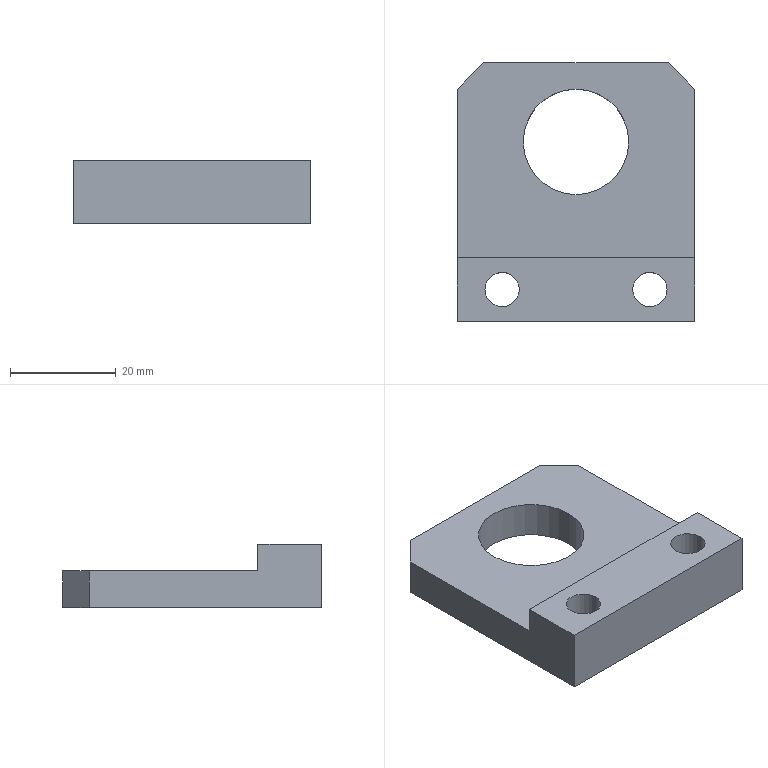Part | STEP file | magnetic tile top shaft cylinder seat 2 | 1 solid | 16 faces | box 45 x 49 x 12 mm | volume 14964 mm3 | plane 10 | cylinder 6 | commonest cylinder face diameters 6.5 x4 20 x2
STEP:
#1=CARTESIAN_POINT('',(0.,0.,0.));
#2=DIRECTION('',(0.,0.,1.));
#3=DIRECTION('',(1.,0.,0.));
#4=AXIS2_PLACEMENT_3D('',#1,#2,#3);
#5=CARTESIAN_POINT('',(10.75,-28.,12.));
#6=VERTEX_POINT('',#5);
#7=CARTESIAN_POINT('',(10.75,-28.,0.));
#8=VERTEX_POINT('',#7);
#9=CARTESIAN_POINT('',(10.75,-28.,12.));
#10=DIRECTION('',(0.,0.,-1.));
#11=VECTOR('',#10,1.);
#12=LINE('',#9,#11);
#13=CARTESIAN_POINT('',(14.,-28.,12.));
#14=DIRECTION('',(0.,0.,-1.));
#15=DIRECTION('',(-1.,0.,0.));
#16=AXIS2_PLACEMENT_3D('',#13,#14,#15);
#17=CYLINDRICAL_SURFACE('',#16,3.25);
#18=CARTESIAN_POINT('',(6.283,0.));
#19=DIRECTION('',(0.,1.));
#20=VECTOR('',#19,1.);
#21=LINE('',#18,#20);
#22=(GEOMETRIC_REPRESENTATION_CONTEXT(2)PARAMETRIC_REPRESENTATION_CONTEXT()REPRESENTATION_CONTEXT('',''));
#23=DEFINITIONAL_REPRESENTATION('',(#21),#22);
#24=PCURVE('',#17,#23);
#25=CARTESIAN_POINT('',(14.,-28.,12.));
#26=DIRECTION('',(0.,0.,-1.));
#27=DIRECTION('',(-1.,0.,0.));
#28=AXIS2_PLACEMENT_3D('',#25,#26,#27);
#29=CYLINDRICAL_SURFACE('',#28,3.25);
#30=CARTESIAN_POINT('',(0.,0.));
#31=DIRECTION('',(0.,1.));
#32=VECTOR('',#31,1.);
#33=LINE('',#30,#32);
#34=(GEOMETRIC_REPRESENTATION_CONTEXT(2)PARAMETRIC_REPRESENTATION_CONTEXT()REPRESENTATION_CONTEXT('',''));
#35=DEFINITIONAL_REPRESENTATION('',(#33),#34);
#36=PCURVE('',#29,#35);
#37=SURFACE_CURVE('',#12,(#24,#36),.PCURVE_S1.);
#38=EDGE_CURVE('',#6,#8,#37,.T.);
#39=ORIENTED_EDGE('',*,*,#38,.T.);
#40=CARTESIAN_POINT('',(17.25,-28.,0.));
#41=VERTEX_POINT('',#40);
#42=CARTESIAN_POINT('',(14.,-28.,0.));
#43=DIRECTION('',(0.,0.,-1.));
#44=DIRECTION('',(-1.,0.,0.));
#45=AXIS2_PLACEMENT_3D('',#42,#43,#44);
#46=CIRCLE('',#45,3.25);
#47=CARTESIAN_POINT('',(0.,12.));
#48=DIRECTION('',(1.,0.));
#49=VECTOR('',#48,1.);
#50=LINE('',#47,#49);
#51=(GEOMETRIC_REPRESENTATION_CONTEXT(2)PARAMETRIC_REPRESENTATION_CONTEXT()REPRESENTATION_CONTEXT('',''));
#52=DEFINITIONAL_REPRESENTATION('',(#50),#51);
#53=PCURVE('',#17,#52);
#54=CARTESIAN_POINT('',(-22.5,-34.,0.));
#55=DIRECTION('',(0.,0.,1.));
#56=DIRECTION('',(1.,0.,0.));
#57=AXIS2_PLACEMENT_3D('',#54,#55,#56);
#58=PLANE('',#57);
#59=CARTESIAN_POINT('',(33.25,6.));
#60=CARTESIAN_POINT('',(33.25,11.629));
#61=CARTESIAN_POINT('',(38.125,8.815));
#62=CARTESIAN_POINT('',(43.,6.));
#63=CARTESIAN_POINT('',(38.125,3.185));
#64=CARTESIAN_POINT('',(33.25,0.3708));
#65=CARTESIAN_POINT('',(33.25,6.));
#66=(BOUNDED_CURVE()B_SPLINE_CURVE(2,(#59,#60,#61,#62,#63,#64,#65),.UNSPECIFIED.,.T.,.F.)B_SPLINE_CURVE_WITH_KNOTS((1,2,2,2,2,1),(-2.094,0.,2.094,4.189,6.283,8.378),.UNSPECIFIED.)CURVE()GEOMETRIC_REPRESENTATION_ITEM()RATIONAL_B_SPLINE_CURVE((1.,0.5,1.,0.5,1.,0.5,1.))REPRESENTATION_ITEM(''));
#67=(GEOMETRIC_REPRESENTATION_CONTEXT(2)PARAMETRIC_REPRESENTATION_CONTEXT()REPRESENTATION_CONTEXT('',''));
#68=DEFINITIONAL_REPRESENTATION('',(#66),#67);
#69=PCURVE('',#58,#68);
#70=SURFACE_CURVE('',#46,(#53,#69),.PCURVE_S1.);
#71=EDGE_CURVE('',#41,#8,#70,.T.);
#72=ORIENTED_EDGE('',*,*,#71,.F.);
#73=CARTESIAN_POINT('',(17.25,-28.,12.));
#74=VERTEX_POINT('',#73);
#75=CARTESIAN_POINT('',(17.25,-28.,12.));
#76=DIRECTION('',(0.,0.,-1.));
#77=VECTOR('',#76,1.);
#78=LINE('',#75,#77);
#79=CARTESIAN_POINT('',(3.142,0.));
#80=DIRECTION('',(0.,1.));
#81=VECTOR('',#80,1.);
#82=LINE('',#79,#81);
#83=(GEOMETRIC_REPRESENTATION_CONTEXT(2)PARAMETRIC_REPRESENTATION_CONTEXT()REPRESENTATION_CONTEXT('',''));
#84=DEFINITIONAL_REPRESENTATION('',(#82),#83);
#85=PCURVE('',#17,#84);
#86=CARTESIAN_POINT('',(3.142,0.));
#87=DIRECTION('',(0.,1.));
#88=VECTOR('',#87,1.);
#89=LINE('',#86,#88);
#90=(GEOMETRIC_REPRESENTATION_CONTEXT(2)PARAMETRIC_REPRESENTATION_CONTEXT()REPRESENTATION_CONTEXT('',''));
#91=DEFINITIONAL_REPRESENTATION('',(#89),#90);
#92=PCURVE('',#29,#91);
#93=SURFACE_CURVE('',#78,(#85,#92),.PCURVE_S1.);
#94=EDGE_CURVE('',#74,#41,#93,.T.);
#95=ORIENTED_EDGE('',*,*,#94,.F.);
#96=CARTESIAN_POINT('',(14.,-28.,12.));
#97=DIRECTION('',(0.,0.,-1.));
#98=DIRECTION('',(-1.,0.,0.));
#99=AXIS2_PLACEMENT_3D('',#96,#97,#98);
#100=CIRCLE('',#99,3.25);
#101=CARTESIAN_POINT('',(0.,0.));
#102=DIRECTION('',(1.,0.));
#103=VECTOR('',#102,1.);
#104=LINE('',#101,#103);
#105=(GEOMETRIC_REPRESENTATION_CONTEXT(2)PARAMETRIC_REPRESENTATION_CONTEXT()REPRESENTATION_CONTEXT('',''));
#106=DEFINITIONAL_REPRESENTATION('',(#104),#105);
#107=PCURVE('',#17,#106);
#108=CARTESIAN_POINT('',(-22.5,-34.,12.));
#109=DIRECTION('',(0.,0.,1.));
#110=DIRECTION('',(1.,0.,0.));
#111=AXIS2_PLACEMENT_3D('',#108,#109,#110);
#112=PLANE('',#111);
#113=CARTESIAN_POINT('',(33.25,6.));
#114=CARTESIAN_POINT('',(33.25,11.629));
#115=CARTESIAN_POINT('',(38.125,8.815));
#116=CARTESIAN_POINT('',(43.,6.));
#117=CARTESIAN_POINT('',(38.125,3.185));
#118=CARTESIAN_POINT('',(33.25,0.3708));
#119=CARTESIAN_POINT('',(33.25,6.));
#120=(BOUNDED_CURVE()B_SPLINE_CURVE(2,(#113,#114,#115,#116,#117,#118,#119),.UNSPECIFIED.,.T.,.F.)B_SPLINE_CURVE_WITH_KNOTS((1,2,2,2,2,1),(-2.094,0.,2.094,4.189,6.283,8.378),.UNSPECIFIED.)CURVE()GEOMETRIC_REPRESENTATION_ITEM()RATIONAL_B_SPLINE_CURVE((1.,0.5,1.,0.5,1.,0.5,1.))REPRESENTATION_ITEM(''));
#121=(GEOMETRIC_REPRESENTATION_CONTEXT(2)PARAMETRIC_REPRESENTATION_CONTEXT()REPRESENTATION_CONTEXT('',''));
#122=DEFINITIONAL_REPRESENTATION('',(#120),#121);
#123=PCURVE('',#112,#122);
#124=SURFACE_CURVE('',#100,(#107,#123),.PCURVE_S1.);
#125=EDGE_CURVE('',#74,#6,#124,.T.);
#126=ORIENTED_EDGE('',*,*,#125,.T.);
#127=EDGE_LOOP('',(#39,#72,#95,#126));
#128=FACE_BOUND('',#127,.F.);
#129=ADVANCED_FACE('',(#128),#17,.F.);
#130=CARTESIAN_POINT('',(-17.25,-28.,12.));
#131=VERTEX_POINT('',#130);
#132=CARTESIAN_POINT('',(-17.25,-28.,0.));
#133=VERTEX_POINT('',#132);
#134=CARTESIAN_POINT('',(-17.25,-28.,12.));
#135=DIRECTION('',(0.,0.,-1.));
#136=VECTOR('',#135,1.);
#137=LINE('',#134,#136);
#138=CARTESIAN_POINT('',(-14.,-28.,12.));
#139=DIRECTION('',(0.,0.,-1.));
#140=DIRECTION('',(-1.,0.,0.));
#141=AXIS2_PLACEMENT_3D('',#138,#139,#140);
#142=CYLINDRICAL_SURFACE('',#141,3.25);
#143=CARTESIAN_POINT('',(6.283,0.));
#144=DIRECTION('',(0.,1.));
#145=VECTOR('',#144,1.);
#146=LINE('',#143,#145);
#147=(GEOMETRIC_REPRESENTATION_CONTEXT(2)PARAMETRIC_REPRESENTATION_CONTEXT()REPRESENTATION_CONTEXT('',''));
#148=DEFINITIONAL_REPRESENTATION('',(#146),#147);
#149=PCURVE('',#142,#148);
#150=CARTESIAN_POINT('',(-14.,-28.,12.));
#151=DIRECTION('',(0.,0.,-1.));
#152=DIRECTION('',(-1.,0.,0.));
#153=AXIS2_PLACEMENT_3D('',#150,#151,#152);
#154=CYLINDRICAL_SURFACE('',#153,3.25);
#155=CARTESIAN_POINT('',(0.,0.));
#156=DIRECTION('',(0.,1.));
#157=VECTOR('',#156,1.);
#158=LINE('',#155,#157);
#159=(GEOMETRIC_REPRESENTATION_CONTEXT(2)PARAMETRIC_REPRESENTATION_CONTEXT()REPRESENTATION_CONTEXT('',''));
#160=DEFINITIONAL_REPRESENTATION('',(#158),#159);
#161=PCURVE('',#154,#160);
#162=SURFACE_CURVE('',#137,(#149,#161),.PCURVE_S1.);
#163=EDGE_CURVE('',#131,#133,#162,.T.);
#164=ORIENTED_EDGE('',*,*,#163,.T.);
#165=CARTESIAN_POINT('',(-10.75,-28.,0.));
#166=VERTEX_POINT('',#165);
#167=CARTESIAN_POINT('',(-14.,-28.,0.));
#168=DIRECTION('',(0.,0.,-1.));
#169=DIRECTION('',(-1.,0.,0.));
#170=AXIS2_PLACEMENT_3D('',#167,#168,#169);
#171=CIRCLE('',#170,3.25);
#172=CARTESIAN_POINT('',(0.,12.));
#173=DIRECTION('',(1.,0.));
#174=VECTOR('',#173,1.);
#175=LINE('',#172,#174);
#176=(GEOMETRIC_REPRESENTATION_CONTEXT(2)PARAMETRIC_REPRESENTATION_CONTEXT()REPRESENTATION_CONTEXT('',''));
#177=DEFINITIONAL_REPRESENTATION('',(#175),#176);
#178=PCURVE('',#142,#177);
#179=CARTESIAN_POINT('',(5.25,6.));
#180=CARTESIAN_POINT('',(5.25,11.629));
#181=CARTESIAN_POINT('',(10.125,8.815));
#182=CARTESIAN_POINT('',(15.,6.));
#183=CARTESIAN_POINT('',(10.125,3.185));
#184=CARTESIAN_POINT('',(5.25,0.3708));
#185=CARTESIAN_POINT('',(5.25,6.));
#186=(BOUNDED_CURVE()B_SPLINE_CURVE(2,(#179,#180,#181,#182,#183,#184,#185),.UNSPECIFIED.,.T.,.F.)B_SPLINE_CURVE_WITH_KNOTS((1,2,2,2,2,1),(-2.094,0.,2.094,4.189,6.283,8.378),.UNSPECIFIED.)CURVE()GEOMETRIC_REPRESENTATION_ITEM()RATIONAL_B_SPLINE_CURVE((1.,0.5,1.,0.5,1.,0.5,1.))REPRESENTATION_ITEM(''));
#187=(GEOMETRIC_REPRESENTATION_CONTEXT(2)PARAMETRIC_REPRESENTATION_CONTEXT()REPRESENTATION_CONTEXT('',''));
#188=DEFINITIONAL_REPRESENTATION('',(#186),#187);
#189=PCURVE('',#58,#188);
#190=SURFACE_CURVE('',#171,(#178,#189),.PCURVE_S1.);
#191=EDGE_CURVE('',#166,#133,#190,.T.);
#192=ORIENTED_EDGE('',*,*,#191,.F.);
#193=CARTESIAN_POINT('',(-10.75,-28.,12.));
#194=VERTEX_POINT('',#193);
#195=CARTESIAN_POINT('',(-10.75,-28.,12.));
#196=DIRECTION('',(0.,0.,-1.));
#197=VECTOR('',#196,1.);
#198=LINE('',#195,#197);
#199=CARTESIAN_POINT('',(3.142,0.));
#200=DIRECTION('',(0.,1.));
#201=VECTOR('',#200,1.);
#202=LINE('',#199,#201);
#203=(GEOMETRIC_REPRESENTATION_CONTEXT(2)PARAMETRIC_REPRESENTATION_CONTEXT()REPRESENTATION_CONTEXT('',''));
#204=DEFINITIONAL_REPRESENTATION('',(#202),#203);
#205=PCURVE('',#142,#204);
#206=CARTESIAN_POINT('',(3.142,0.));
#207=DIRECTION('',(0.,1.));
#208=VECTOR('',#207,1.);
#209=LINE('',#206,#208);
#210=(GEOMETRIC_REPRESENTATION_CONTEXT(2)PARAMETRIC_REPRESENTATION_CONTEXT()REPRESENTATION_CONTEXT('',''));
#211=DEFINITIONAL_REPRESENTATION('',(#209),#210);
#212=PCURVE('',#154,#211);
#213=SURFACE_CURVE('',#198,(#205,#212),.PCURVE_S1.);
#214=EDGE_CURVE('',#194,#166,#213,.T.);
#215=ORIENTED_EDGE('',*,*,#214,.F.);
#216=CARTESIAN_POINT('',(-14.,-28.,12.));
#217=DIRECTION('',(0.,0.,-1.));
#218=DIRECTION('',(-1.,0.,0.));
#219=AXIS2_PLACEMENT_3D('',#216,#217,#218);
#220=CIRCLE('',#219,3.25);
#221=CARTESIAN_POINT('',(0.,0.));
#222=DIRECTION('',(1.,0.));
#223=VECTOR('',#222,1.);
#224=LINE('',#221,#223);
#225=(GEOMETRIC_REPRESENTATION_CONTEXT(2)PARAMETRIC_REPRESENTATION_CONTEXT()REPRESENTATION_CONTEXT('',''));
#226=DEFINITIONAL_REPRESENTATION('',(#224),#225);
#227=PCURVE('',#142,#226);
#228=CARTESIAN_POINT('',(5.25,6.));
#229=CARTESIAN_POINT('',(5.25,11.629));
#230=CARTESIAN_POINT('',(10.125,8.815));
#231=CARTESIAN_POINT('',(15.,6.));
#232=CARTESIAN_POINT('',(10.125,3.185));
#233=CARTESIAN_POINT('',(5.25,0.3708));
#234=CARTESIAN_POINT('',(5.25,6.));
#235=(BOUNDED_CURVE()B_SPLINE_CURVE(2,(#228,#229,#230,#231,#232,#233,#234),.UNSPECIFIED.,.T.,.F.)B_SPLINE_CURVE_WITH_KNOTS((1,2,2,2,2,1),(-2.094,0.,2.094,4.189,6.283,8.378),.UNSPECIFIED.)CURVE()GEOMETRIC_REPRESENTATION_ITEM()RATIONAL_B_SPLINE_CURVE((1.,0.5,1.,0.5,1.,0.5,1.))REPRESENTATION_ITEM(''));
#236=(GEOMETRIC_REPRESENTATION_CONTEXT(2)PARAMETRIC_REPRESENTATION_CONTEXT()REPRESENTATION_CONTEXT('',''));
#237=DEFINITIONAL_REPRESENTATION('',(#235),#236);
#238=PCURVE('',#112,#237);
#239=SURFACE_CURVE('',#220,(#227,#238),.PCURVE_S1.);
#240=EDGE_CURVE('',#194,#131,#239,.T.);
#241=ORIENTED_EDGE('',*,*,#240,.T.);
#242=EDGE_LOOP('',(#164,#192,#215,#241));
#243=FACE_BOUND('',#242,.F.);
#244=ADVANCED_FACE('',(#243),#142,.F.);
#245=CARTESIAN_POINT('',(-10.,0.,7.));
#246=VERTEX_POINT('',#245);
#247=CARTESIAN_POINT('',(-10.,0.,0.));
#248=VERTEX_POINT('',#247);
#249=CARTESIAN_POINT('',(-10.,0.,12.));
#250=DIRECTION('',(0.,0.,-1.));
#251=VECTOR('',#250,1.);
#252=LINE('',#249,#251);
#253=CARTESIAN_POINT('',(0.,0.,12.));
#254=DIRECTION('',(0.,0.,-1.));
#255=DIRECTION('',(-1.,0.,0.));
#256=AXIS2_PLACEMENT_3D('',#253,#254,#255);
#257=CYLINDRICAL_SURFACE('',#256,10.);
#258=CARTESIAN_POINT('',(6.283,0.));
#259=DIRECTION('',(0.,1.));
#260=VECTOR('',#259,1.);
#261=LINE('',#258,#260);
#262=(GEOMETRIC_REPRESENTATION_CONTEXT(2)PARAMETRIC_REPRESENTATION_CONTEXT()REPRESENTATION_CONTEXT('',''));
#263=DEFINITIONAL_REPRESENTATION('',(#261),#262);
#264=PCURVE('',#257,#263);
#265=CARTESIAN_POINT('',(0.,0.,12.));
#266=DIRECTION('',(0.,0.,-1.));
#267=DIRECTION('',(-1.,0.,0.));
#268=AXIS2_PLACEMENT_3D('',#265,#266,#267);
#269=CYLINDRICAL_SURFACE('',#268,10.);
#270=CARTESIAN_POINT('',(0.,0.));
#271=DIRECTION('',(0.,1.));
#272=VECTOR('',#271,1.);
#273=LINE('',#270,#272);
#274=(GEOMETRIC_REPRESENTATION_CONTEXT(2)PARAMETRIC_REPRESENTATION_CONTEXT()REPRESENTATION_CONTEXT('',''));
#275=DEFINITIONAL_REPRESENTATION('',(#273),#274);
#276=PCURVE('',#269,#275);
#277=SURFACE_CURVE('',#252,(#264,#276),.PCURVE_S1.);
#278=EDGE_CURVE('',#246,#248,#277,.T.);
#279=ORIENTED_EDGE('',*,*,#278,.T.);
#280=CARTESIAN_POINT('',(10.,0.,0.));
#281=VERTEX_POINT('',#280);
#282=CARTESIAN_POINT('',(0.,0.,0.));
#283=DIRECTION('',(0.,0.,1.));
#284=DIRECTION('',(1.,0.,0.));
#285=AXIS2_PLACEMENT_3D('',#282,#283,#284);
#286=CIRCLE('',#285,10.);
#287=CARTESIAN_POINT('',(9.425,12.));
#288=DIRECTION('',(-1.,0.));
#289=VECTOR('',#288,1.);
#290=LINE('',#287,#289);
#291=(GEOMETRIC_REPRESENTATION_CONTEXT(2)PARAMETRIC_REPRESENTATION_CONTEXT()REPRESENTATION_CONTEXT('',''));
#292=DEFINITIONAL_REPRESENTATION('',(#290),#291);
#293=PCURVE('',#257,#292);
#294=CARTESIAN_POINT('',(22.5,34.));
#295=DIRECTION('',(1.,0.));
#296=AXIS2_PLACEMENT_2D('',#294,#295);
#297=CIRCLE('',#296,10.);
#298=(GEOMETRIC_REPRESENTATION_CONTEXT(2)PARAMETRIC_REPRESENTATION_CONTEXT()REPRESENTATION_CONTEXT('',''));
#299=DEFINITIONAL_REPRESENTATION('',(#297),#298);
#300=PCURVE('',#58,#299);
#301=SURFACE_CURVE('',#286,(#293,#300),.PCURVE_S1.);
#302=EDGE_CURVE('',#248,#281,#301,.T.);
#303=ORIENTED_EDGE('',*,*,#302,.T.);
#304=CARTESIAN_POINT('',(10.,0.,7.));
#305=VERTEX_POINT('',#304);
#306=CARTESIAN_POINT('',(10.,0.,12.));
#307=DIRECTION('',(0.,0.,-1.));
#308=VECTOR('',#307,1.);
#309=LINE('',#306,#308);
#310=CARTESIAN_POINT('',(3.142,0.));
#311=DIRECTION('',(0.,1.));
#312=VECTOR('',#311,1.);
#313=LINE('',#310,#312);
#314=(GEOMETRIC_REPRESENTATION_CONTEXT(2)PARAMETRIC_REPRESENTATION_CONTEXT()REPRESENTATION_CONTEXT('',''));
#315=DEFINITIONAL_REPRESENTATION('',(#313),#314);
#316=PCURVE('',#257,#315);
#317=CARTESIAN_POINT('',(3.142,0.));
#318=DIRECTION('',(0.,1.));
#319=VECTOR('',#318,1.);
#320=LINE('',#317,#319);
#321=(GEOMETRIC_REPRESENTATION_CONTEXT(2)PARAMETRIC_REPRESENTATION_CONTEXT()REPRESENTATION_CONTEXT('',''));
#322=DEFINITIONAL_REPRESENTATION('',(#320),#321);
#323=PCURVE('',#269,#322);
#324=SURFACE_CURVE('',#309,(#316,#323),.PCURVE_S1.);
#325=EDGE_CURVE('',#305,#281,#324,.T.);
#326=ORIENTED_EDGE('',*,*,#325,.F.);
#327=CARTESIAN_POINT('',(0.,0.,7.));
#328=DIRECTION('',(0.,0.,1.));
#329=DIRECTION('',(1.,0.,0.));
#330=AXIS2_PLACEMENT_3D('',#327,#328,#329);
#331=CIRCLE('',#330,10.);
#332=CARTESIAN_POINT('',(9.425,5.));
#333=DIRECTION('',(-1.,0.));
#334=VECTOR('',#333,1.);
#335=LINE('',#332,#334);
#336=(GEOMETRIC_REPRESENTATION_CONTEXT(2)PARAMETRIC_REPRESENTATION_CONTEXT()REPRESENTATION_CONTEXT('',''));
#337=DEFINITIONAL_REPRESENTATION('',(#335),#336);
#338=PCURVE('',#257,#337);
#339=CARTESIAN_POINT('',(-34.163,-22.,7.));
#340=DIRECTION('',(0.,0.,1.));
#341=DIRECTION('',(1.,0.,0.));
#342=AXIS2_PLACEMENT_3D('',#339,#340,#341);
#343=PLANE('',#342);
#344=CARTESIAN_POINT('',(34.163,22.));
#345=DIRECTION('',(1.,0.));
#346=AXIS2_PLACEMENT_2D('',#344,#345);
#347=CIRCLE('',#346,10.);
#348=(GEOMETRIC_REPRESENTATION_CONTEXT(2)PARAMETRIC_REPRESENTATION_CONTEXT()REPRESENTATION_CONTEXT('',''));
#349=DEFINITIONAL_REPRESENTATION('',(#347),#348);
#350=PCURVE('',#343,#349);
#351=SURFACE_CURVE('',#331,(#338,#350),.PCURVE_S1.);
#352=EDGE_CURVE('',#246,#305,#351,.T.);
#353=ORIENTED_EDGE('',*,*,#352,.F.);
#354=EDGE_LOOP('',(#279,#303,#326,#353));
#355=FACE_BOUND('',#354,.F.);
#356=ADVANCED_FACE('',(#355),#257,.F.);
#357=CARTESIAN_POINT('',(17.5,15.,7.));
#358=VERTEX_POINT('',#357);
#359=CARTESIAN_POINT('',(-17.5,15.,7.));
#360=VERTEX_POINT('',#359);
#361=CARTESIAN_POINT('',(-22.5,15.,7.));
#362=DIRECTION('',(-1.,0.,0.));
#363=VECTOR('',#362,1.);
#364=LINE('',#361,#363);
#365=CARTESIAN_POINT('',(-22.5,15.,12.));
#366=DIRECTION('',(0.,-1.,0.));
#367=DIRECTION('',(0.,0.,-1.));
#368=AXIS2_PLACEMENT_3D('',#365,#366,#367);
#369=PLANE('',#368);
#370=CARTESIAN_POINT('',(5.,0.));
#371=DIRECTION('',(0.,-1.));
#372=VECTOR('',#371,1.);
#373=LINE('',#370,#372);
#374=(GEOMETRIC_REPRESENTATION_CONTEXT(2)PARAMETRIC_REPRESENTATION_CONTEXT()REPRESENTATION_CONTEXT('',''));
#375=DEFINITIONAL_REPRESENTATION('',(#373),#374);
#376=PCURVE('',#369,#375);
#377=CARTESIAN_POINT('',(11.663,37.));
#378=DIRECTION('',(-1.,0.));
#379=VECTOR('',#378,1.);
#380=LINE('',#377,#379);
#381=(GEOMETRIC_REPRESENTATION_CONTEXT(2)PARAMETRIC_REPRESENTATION_CONTEXT()REPRESENTATION_CONTEXT('',''));
#382=DEFINITIONAL_REPRESENTATION('',(#380),#381);
#383=PCURVE('',#343,#382);
#384=SURFACE_CURVE('',#364,(#376,#383),.PCURVE_S1.);
#385=EDGE_CURVE('',#358,#360,#384,.T.);
#386=ORIENTED_EDGE('',*,*,#385,.F.);
#387=CARTESIAN_POINT('',(17.5,15.,0.));
#388=VERTEX_POINT('',#387);
#389=CARTESIAN_POINT('',(17.5,15.,12.));
#390=DIRECTION('',(0.,0.,-1.));
#391=VECTOR('',#390,1.);
#392=LINE('',#389,#391);
#393=CARTESIAN_POINT('',(0.,40.));
#394=DIRECTION('',(1.,0.));
#395=VECTOR('',#394,1.);
#396=LINE('',#393,#395);
#397=(GEOMETRIC_REPRESENTATION_CONTEXT(2)PARAMETRIC_REPRESENTATION_CONTEXT()REPRESENTATION_CONTEXT('',''));
#398=DEFINITIONAL_REPRESENTATION('',(#396),#397);
#399=PCURVE('',#369,#398);
#400=CARTESIAN_POINT('',(17.5,15.,12.));
#401=DIRECTION('',(-0.7071,-0.7071,0.));
#402=DIRECTION('',(0.7071,-0.7071,0.));
#403=AXIS2_PLACEMENT_3D('',#400,#401,#402);
#404=PLANE('',#403);
#405=CARTESIAN_POINT('',(0.,0.));
#406=DIRECTION('',(0.,-1.));
#407=VECTOR('',#406,1.);
#408=LINE('',#405,#407);
#409=(GEOMETRIC_REPRESENTATION_CONTEXT(2)PARAMETRIC_REPRESENTATION_CONTEXT()REPRESENTATION_CONTEXT('',''));
#410=DEFINITIONAL_REPRESENTATION('',(#408),#409);
#411=PCURVE('',#404,#410);
#412=SURFACE_CURVE('',#392,(#399,#411),.PCURVE_S1.);
#413=EDGE_CURVE('',#358,#388,#412,.T.);
#414=ORIENTED_EDGE('',*,*,#413,.T.);
#415=CARTESIAN_POINT('',(-17.5,15.,0.));
#416=VERTEX_POINT('',#415);
#417=CARTESIAN_POINT('',(-22.5,15.,0.));
#418=DIRECTION('',(-1.,0.,0.));
#419=VECTOR('',#418,1.);
#420=LINE('',#417,#419);
#421=CARTESIAN_POINT('',(12.,0.));
#422=DIRECTION('',(0.,-1.));
#423=VECTOR('',#422,1.);
#424=LINE('',#421,#423);
#425=(GEOMETRIC_REPRESENTATION_CONTEXT(2)PARAMETRIC_REPRESENTATION_CONTEXT()REPRESENTATION_CONTEXT('',''));
#426=DEFINITIONAL_REPRESENTATION('',(#424),#425);
#427=PCURVE('',#369,#426);
#428=CARTESIAN_POINT('',(0.,49.));
#429=DIRECTION('',(-1.,0.));
#430=VECTOR('',#429,1.);
#431=LINE('',#428,#430);
#432=(GEOMETRIC_REPRESENTATION_CONTEXT(2)PARAMETRIC_REPRESENTATION_CONTEXT()REPRESENTATION_CONTEXT('',''));
#433=DEFINITIONAL_REPRESENTATION('',(#431),#432);
#434=PCURVE('',#58,#433);
#435=SURFACE_CURVE('',#420,(#427,#434),.PCURVE_S1.);
#436=EDGE_CURVE('',#388,#416,#435,.T.);
#437=ORIENTED_EDGE('',*,*,#436,.T.);
#438=CARTESIAN_POINT('',(-17.5,15.,12.));
#439=DIRECTION('',(0.,0.,1.));
#440=VECTOR('',#439,1.);
#441=LINE('',#438,#440);
#442=CARTESIAN_POINT('',(0.,5.));
#443=DIRECTION('',(-1.,0.));
#444=VECTOR('',#443,1.);
#445=LINE('',#442,#444);
#446=(GEOMETRIC_REPRESENTATION_CONTEXT(2)PARAMETRIC_REPRESENTATION_CONTEXT()REPRESENTATION_CONTEXT('',''));
#447=DEFINITIONAL_REPRESENTATION('',(#445),#446);
#448=PCURVE('',#369,#447);
#449=CARTESIAN_POINT('',(-22.5,10.,12.));
#450=DIRECTION('',(0.7071,-0.7071,0.));
#451=DIRECTION('',(0.7071,0.7071,0.));
#452=AXIS2_PLACEMENT_3D('',#449,#450,#451);
#453=PLANE('',#452);
#454=CARTESIAN_POINT('',(7.071,0.));
#455=DIRECTION('',(0.,1.));
#456=VECTOR('',#455,1.);
#457=LINE('',#454,#456);
#458=(GEOMETRIC_REPRESENTATION_CONTEXT(2)PARAMETRIC_REPRESENTATION_CONTEXT()REPRESENTATION_CONTEXT('',''));
#459=DEFINITIONAL_REPRESENTATION('',(#457),#458);
#460=PCURVE('',#453,#459);
#461=SURFACE_CURVE('',#441,(#448,#460),.PCURVE_S1.);
#462=EDGE_CURVE('',#416,#360,#461,.T.);
#463=ORIENTED_EDGE('',*,*,#462,.T.);
#464=EDGE_LOOP('',(#386,#414,#437,#463));
#465=FACE_BOUND('',#464,.T.);
#466=ADVANCED_FACE('',(#465),#369,.F.);
#467=CARTESIAN_POINT('',(0.,0.,0.));
#468=DIRECTION('',(0.,0.,1.));
#469=DIRECTION('',(1.,0.,0.));
#470=AXIS2_PLACEMENT_3D('',#467,#468,#469);
#471=CIRCLE('',#470,10.);
#472=CARTESIAN_POINT('',(3.142,12.));
#473=DIRECTION('',(-1.,0.));
#474=VECTOR('',#473,1.);
#475=LINE('',#472,#474);
#476=(GEOMETRIC_REPRESENTATION_CONTEXT(2)PARAMETRIC_REPRESENTATION_CONTEXT()REPRESENTATION_CONTEXT('',''));
#477=DEFINITIONAL_REPRESENTATION('',(#475),#476);
#478=PCURVE('',#269,#477);
#479=CARTESIAN_POINT('',(22.5,34.));
#480=DIRECTION('',(1.,0.));
#481=AXIS2_PLACEMENT_2D('',#479,#480);
#482=CIRCLE('',#481,10.);
#483=(GEOMETRIC_REPRESENTATION_CONTEXT(2)PARAMETRIC_REPRESENTATION_CONTEXT()REPRESENTATION_CONTEXT('',''));
#484=DEFINITIONAL_REPRESENTATION('',(#482),#483);
#485=PCURVE('',#58,#484);
#486=SURFACE_CURVE('',#471,(#478,#485),.PCURVE_S1.);
#487=EDGE_CURVE('',#281,#248,#486,.T.);
#488=ORIENTED_EDGE('',*,*,#487,.T.);
#489=ORIENTED_EDGE('',*,*,#278,.F.);
#490=CARTESIAN_POINT('',(0.,0.,7.));
#491=DIRECTION('',(0.,0.,1.));
#492=DIRECTION('',(1.,0.,0.));
#493=AXIS2_PLACEMENT_3D('',#490,#491,#492);
#494=CIRCLE('',#493,10.);
#495=CARTESIAN_POINT('',(3.142,5.));
#496=DIRECTION('',(-1.,0.));
#497=VECTOR('',#496,1.);
#498=LINE('',#495,#497);
#499=(GEOMETRIC_REPRESENTATION_CONTEXT(2)PARAMETRIC_REPRESENTATION_CONTEXT()REPRESENTATION_CONTEXT('',''));
#500=DEFINITIONAL_REPRESENTATION('',(#498),#499);
#501=PCURVE('',#269,#500);
#502=CARTESIAN_POINT('',(34.163,22.));
#503=DIRECTION('',(1.,0.));
#504=AXIS2_PLACEMENT_2D('',#502,#503);
#505=CIRCLE('',#504,10.);
#506=(GEOMETRIC_REPRESENTATION_CONTEXT(2)PARAMETRIC_REPRESENTATION_CONTEXT()REPRESENTATION_CONTEXT('',''));
#507=DEFINITIONAL_REPRESENTATION('',(#505),#506);
#508=PCURVE('',#343,#507);
#509=SURFACE_CURVE('',#494,(#501,#508),.PCURVE_S1.);
#510=EDGE_CURVE('',#305,#246,#509,.T.);
#511=ORIENTED_EDGE('',*,*,#510,.F.);
#512=ORIENTED_EDGE('',*,*,#325,.T.);
#513=EDGE_LOOP('',(#488,#489,#511,#512));
#514=FACE_BOUND('',#513,.F.);
#515=ADVANCED_FACE('',(#514),#269,.F.);
#516=CARTESIAN_POINT('',(-22.5,10.,7.));
#517=VERTEX_POINT('',#516);
#518=CARTESIAN_POINT('',(-22.5,10.,0.));
#519=VERTEX_POINT('',#518);
#520=CARTESIAN_POINT('',(-22.5,10.,12.));
#521=DIRECTION('',(0.,0.,-1.));
#522=VECTOR('',#521,1.);
#523=LINE('',#520,#522);
#524=CARTESIAN_POINT('',(0.,0.));
#525=DIRECTION('',(0.,-1.));
#526=VECTOR('',#525,1.);
#527=LINE('',#524,#526);
#528=(GEOMETRIC_REPRESENTATION_CONTEXT(2)PARAMETRIC_REPRESENTATION_CONTEXT()REPRESENTATION_CONTEXT('',''));
#529=DEFINITIONAL_REPRESENTATION('',(#527),#528);
#530=PCURVE('',#453,#529);
#531=CARTESIAN_POINT('',(-22.5,15.,12.));
#532=DIRECTION('',(1.,0.,0.));
#533=DIRECTION('',(0.,1.,0.));
#534=AXIS2_PLACEMENT_3D('',#531,#532,#533);
#535=PLANE('',#534);
#536=CARTESIAN_POINT('',(-5.,0.));
#537=DIRECTION('',(0.,-1.));
#538=VECTOR('',#537,1.);
#539=LINE('',#536,#538);
#540=(GEOMETRIC_REPRESENTATION_CONTEXT(2)PARAMETRIC_REPRESENTATION_CONTEXT()REPRESENTATION_CONTEXT('',''));
#541=DEFINITIONAL_REPRESENTATION('',(#539),#540);
#542=PCURVE('',#535,#541);
#543=SURFACE_CURVE('',#523,(#530,#542),.PCURVE_S1.);
#544=EDGE_CURVE('',#517,#519,#543,.T.);
#545=ORIENTED_EDGE('',*,*,#544,.F.);
#546=CARTESIAN_POINT('',(-22.5,10.,7.));
#547=DIRECTION('',(0.7071,0.7071,0.));
#548=VECTOR('',#547,1.);
#549=LINE('',#546,#548);
#550=CARTESIAN_POINT('',(0.,-5.));
#551=DIRECTION('',(1.,0.));
#552=VECTOR('',#551,1.);
#553=LINE('',#550,#552);
#554=(GEOMETRIC_REPRESENTATION_CONTEXT(2)PARAMETRIC_REPRESENTATION_CONTEXT()REPRESENTATION_CONTEXT('',''));
#555=DEFINITIONAL_REPRESENTATION('',(#553),#554);
#556=PCURVE('',#453,#555);
#557=CARTESIAN_POINT('',(11.663,32.));
#558=DIRECTION('',(0.7071,0.7071));
#559=VECTOR('',#558,1.);
#560=LINE('',#557,#559);
#561=(GEOMETRIC_REPRESENTATION_CONTEXT(2)PARAMETRIC_REPRESENTATION_CONTEXT()REPRESENTATION_CONTEXT('',''));
#562=DEFINITIONAL_REPRESENTATION('',(#560),#561);
#563=PCURVE('',#343,#562);
#564=SURFACE_CURVE('',#549,(#556,#563),.PCURVE_S1.);
#565=EDGE_CURVE('',#517,#360,#564,.T.);
#566=ORIENTED_EDGE('',*,*,#565,.T.);
#567=ORIENTED_EDGE('',*,*,#462,.F.);
#568=CARTESIAN_POINT('',(-22.5,10.,0.));
#569=DIRECTION('',(0.7071,0.7071,0.));
#570=VECTOR('',#569,1.);
#571=LINE('',#568,#570);
#572=CARTESIAN_POINT('',(0.,-12.));
#573=DIRECTION('',(1.,0.));
#574=VECTOR('',#573,1.);
#575=LINE('',#572,#574);
#576=(GEOMETRIC_REPRESENTATION_CONTEXT(2)PARAMETRIC_REPRESENTATION_CONTEXT()REPRESENTATION_CONTEXT('',''));
#577=DEFINITIONAL_REPRESENTATION('',(#575),#576);
#578=PCURVE('',#453,#577);
#579=CARTESIAN_POINT('',(0.,44.));
#580=DIRECTION('',(0.7071,0.7071));
#581=VECTOR('',#580,1.);
#582=LINE('',#579,#581);
#583=(GEOMETRIC_REPRESENTATION_CONTEXT(2)PARAMETRIC_REPRESENTATION_CONTEXT()REPRESENTATION_CONTEXT('',''));
#584=DEFINITIONAL_REPRESENTATION('',(#582),#583);
#585=PCURVE('',#58,#584);
#586=SURFACE_CURVE('',#571,(#578,#585),.PCURVE_S1.);
#587=EDGE_CURVE('',#519,#416,#586,.T.);
#588=ORIENTED_EDGE('',*,*,#587,.F.);
#589=EDGE_LOOP('',(#545,#566,#567,#588));
#590=FACE_BOUND('',#589,.T.);
#591=ADVANCED_FACE('',(#590),#453,.F.);
#592=ORIENTED_EDGE('',*,*,#413,.F.);
#593=CARTESIAN_POINT('',(22.5,10.,7.));
#594=VERTEX_POINT('',#593);
#595=CARTESIAN_POINT('',(17.5,15.,7.));
#596=DIRECTION('',(0.7071,-0.7071,0.));
#597=VECTOR('',#596,1.);
#598=LINE('',#595,#597);
#599=CARTESIAN_POINT('',(0.,-5.));
#600=DIRECTION('',(1.,0.));
#601=VECTOR('',#600,1.);
#602=LINE('',#599,#601);
#603=(GEOMETRIC_REPRESENTATION_CONTEXT(2)PARAMETRIC_REPRESENTATION_CONTEXT()REPRESENTATION_CONTEXT('',''));
#604=DEFINITIONAL_REPRESENTATION('',(#602),#603);
#605=PCURVE('',#404,#604);
#606=CARTESIAN_POINT('',(51.663,37.));
#607=DIRECTION('',(0.7071,-0.7071));
#608=VECTOR('',#607,1.);
#609=LINE('',#606,#608);
#610=(GEOMETRIC_REPRESENTATION_CONTEXT(2)PARAMETRIC_REPRESENTATION_CONTEXT()REPRESENTATION_CONTEXT('',''));
#611=DEFINITIONAL_REPRESENTATION('',(#609),#610);
#612=PCURVE('',#343,#611);
#613=SURFACE_CURVE('',#598,(#605,#612),.PCURVE_S1.);
#614=EDGE_CURVE('',#358,#594,#613,.T.);
#615=ORIENTED_EDGE('',*,*,#614,.T.);
#616=CARTESIAN_POINT('',(22.5,10.,0.));
#617=VERTEX_POINT('',#616);
#618=CARTESIAN_POINT('',(22.5,10.,12.));
#619=DIRECTION('',(0.,0.,1.));
#620=VECTOR('',#619,1.);
#621=LINE('',#618,#620);
#622=CARTESIAN_POINT('',(7.071,0.));
#623=DIRECTION('',(0.,1.));
#624=VECTOR('',#623,1.);
#625=LINE('',#622,#624);
#626=(GEOMETRIC_REPRESENTATION_CONTEXT(2)PARAMETRIC_REPRESENTATION_CONTEXT()REPRESENTATION_CONTEXT('',''));
#627=DEFINITIONAL_REPRESENTATION('',(#625),#626);
#628=PCURVE('',#404,#627);
#629=CARTESIAN_POINT('',(22.5,15.,12.));
#630=DIRECTION('',(-1.,0.,0.));
#631=DIRECTION('',(0.,-1.,0.));
#632=AXIS2_PLACEMENT_3D('',#629,#630,#631);
#633=PLANE('',#632);
#634=CARTESIAN_POINT('',(5.,0.));
#635=DIRECTION('',(0.,1.));
#636=VECTOR('',#635,1.);
#637=LINE('',#634,#636);
#638=(GEOMETRIC_REPRESENTATION_CONTEXT(2)PARAMETRIC_REPRESENTATION_CONTEXT()REPRESENTATION_CONTEXT('',''));
#639=DEFINITIONAL_REPRESENTATION('',(#637),#638);
#640=PCURVE('',#633,#639);
#641=SURFACE_CURVE('',#621,(#628,#640),.PCURVE_S1.);
#642=EDGE_CURVE('',#617,#594,#641,.T.);
#643=ORIENTED_EDGE('',*,*,#642,.F.);
#644=CARTESIAN_POINT('',(17.5,15.,0.));
#645=DIRECTION('',(0.7071,-0.7071,0.));
#646=VECTOR('',#645,1.);
#647=LINE('',#644,#646);
#648=CARTESIAN_POINT('',(0.,-12.));
#649=DIRECTION('',(1.,0.));
#650=VECTOR('',#649,1.);
#651=LINE('',#648,#650);
#652=(GEOMETRIC_REPRESENTATION_CONTEXT(2)PARAMETRIC_REPRESENTATION_CONTEXT()REPRESENTATION_CONTEXT('',''));
#653=DEFINITIONAL_REPRESENTATION('',(#651),#652);
#654=PCURVE('',#404,#653);
#655=CARTESIAN_POINT('',(40.,49.));
#656=DIRECTION('',(0.7071,-0.7071));
#657=VECTOR('',#656,1.);
#658=LINE('',#655,#657);
#659=(GEOMETRIC_REPRESENTATION_CONTEXT(2)PARAMETRIC_REPRESENTATION_CONTEXT()REPRESENTATION_CONTEXT('',''));
#660=DEFINITIONAL_REPRESENTATION('',(#658),#659);
#661=PCURVE('',#58,#660);
#662=SURFACE_CURVE('',#647,(#654,#661),.PCURVE_S1.);
#663=EDGE_CURVE('',#388,#617,#662,.T.);
#664=ORIENTED_EDGE('',*,*,#663,.F.);
#665=EDGE_LOOP('',(#592,#615,#643,#664));
#666=FACE_BOUND('',#665,.T.);
#667=ADVANCED_FACE('',(#666),#404,.F.);
#668=CARTESIAN_POINT('',(14.,-28.,12.));
#669=DIRECTION('',(0.,0.,-1.));
#670=DIRECTION('',(-1.,0.,0.));
#671=AXIS2_PLACEMENT_3D('',#668,#669,#670);
#672=CIRCLE('',#671,3.25);
#673=CARTESIAN_POINT('',(33.25,6.));
#674=CARTESIAN_POINT('',(33.25,11.629));
#675=CARTESIAN_POINT('',(38.125,8.815));
#676=CARTESIAN_POINT('',(43.,6.));
#677=CARTESIAN_POINT('',(38.125,3.185));
#678=CARTESIAN_POINT('',(33.25,0.3708));
#679=CARTESIAN_POINT('',(33.25,6.));
#680=(BOUNDED_CURVE()B_SPLINE_CURVE(2,(#673,#674,#675,#676,#677,#678,#679),.UNSPECIFIED.,.T.,.F.)B_SPLINE_CURVE_WITH_KNOTS((1,2,2,2,2,1),(-2.094,0.,2.094,4.189,6.283,8.378),.UNSPECIFIED.)CURVE()GEOMETRIC_REPRESENTATION_ITEM()RATIONAL_B_SPLINE_CURVE((1.,0.5,1.,0.5,1.,0.5,1.))REPRESENTATION_ITEM(''));
#681=(GEOMETRIC_REPRESENTATION_CONTEXT(2)PARAMETRIC_REPRESENTATION_CONTEXT()REPRESENTATION_CONTEXT('',''));
#682=DEFINITIONAL_REPRESENTATION('',(#680),#681);
#683=PCURVE('',#112,#682);
#684=CARTESIAN_POINT('',(0.,0.));
#685=DIRECTION('',(1.,0.));
#686=VECTOR('',#685,1.);
#687=LINE('',#684,#686);
#688=(GEOMETRIC_REPRESENTATION_CONTEXT(2)PARAMETRIC_REPRESENTATION_CONTEXT()REPRESENTATION_CONTEXT('',''));
#689=DEFINITIONAL_REPRESENTATION('',(#687),#688);
#690=PCURVE('',#29,#689);
#691=SURFACE_CURVE('',#672,(#683,#690),.PCURVE_S1.);
#692=EDGE_CURVE('',#6,#74,#691,.T.);
#693=ORIENTED_EDGE('',*,*,#692,.T.);
#694=ORIENTED_EDGE('',*,*,#125,.T.);
#695=EDGE_LOOP('',(#693,#694));
#696=FACE_BOUND('',#695,.T.);
#697=CARTESIAN_POINT('',(-14.,-28.,12.));
#698=DIRECTION('',(0.,0.,-1.));
#699=DIRECTION('',(-1.,0.,0.));
#700=AXIS2_PLACEMENT_3D('',#697,#698,#699);
#701=CIRCLE('',#700,3.25);
#702=CARTESIAN_POINT('',(5.25,6.));
#703=CARTESIAN_POINT('',(5.25,11.629));
#704=CARTESIAN_POINT('',(10.125,8.815));
#705=CARTESIAN_POINT('',(15.,6.));
#706=CARTESIAN_POINT('',(10.125,3.185));
#707=CARTESIAN_POINT('',(5.25,0.3708));
#708=CARTESIAN_POINT('',(5.25,6.));
#709=(BOUNDED_CURVE()B_SPLINE_CURVE(2,(#702,#703,#704,#705,#706,#707,#708),.UNSPECIFIED.,.T.,.F.)B_SPLINE_CURVE_WITH_KNOTS((1,2,2,2,2,1),(-2.094,0.,2.094,4.189,6.283,8.378),.UNSPECIFIED.)CURVE()GEOMETRIC_REPRESENTATION_ITEM()RATIONAL_B_SPLINE_CURVE((1.,0.5,1.,0.5,1.,0.5,1.))REPRESENTATION_ITEM(''));
#710=(GEOMETRIC_REPRESENTATION_CONTEXT(2)PARAMETRIC_REPRESENTATION_CONTEXT()REPRESENTATION_CONTEXT('',''));
#711=DEFINITIONAL_REPRESENTATION('',(#709),#710);
#712=PCURVE('',#112,#711);
#713=CARTESIAN_POINT('',(0.,0.));
#714=DIRECTION('',(1.,0.));
#715=VECTOR('',#714,1.);
#716=LINE('',#713,#715);
#717=(GEOMETRIC_REPRESENTATION_CONTEXT(2)PARAMETRIC_REPRESENTATION_CONTEXT()REPRESENTATION_CONTEXT('',''));
#718=DEFINITIONAL_REPRESENTATION('',(#716),#717);
#719=PCURVE('',#154,#718);
#720=SURFACE_CURVE('',#701,(#712,#719),.PCURVE_S1.);
#721=EDGE_CURVE('',#131,#194,#720,.T.);
#722=ORIENTED_EDGE('',*,*,#721,.T.);
#723=ORIENTED_EDGE('',*,*,#240,.T.);
#724=EDGE_LOOP('',(#722,#723));
#725=FACE_BOUND('',#724,.T.);
#726=CARTESIAN_POINT('',(-22.5,-22.,12.));
#727=VERTEX_POINT('',#726);
#728=CARTESIAN_POINT('',(22.5,-22.,12.));
#729=VERTEX_POINT('',#728);
#730=CARTESIAN_POINT('',(-34.163,-22.,12.));
#731=DIRECTION('',(1.,0.,0.));
#732=VECTOR('',#731,1.);
#733=LINE('',#730,#732);
#734=CARTESIAN_POINT('',(-11.663,12.));
#735=DIRECTION('',(1.,0.));
#736=VECTOR('',#735,1.);
#737=LINE('',#734,#736);
#738=(GEOMETRIC_REPRESENTATION_CONTEXT(2)PARAMETRIC_REPRESENTATION_CONTEXT()REPRESENTATION_CONTEXT('',''));
#739=DEFINITIONAL_REPRESENTATION('',(#737),#738);
#740=PCURVE('',#112,#739);
#741=CARTESIAN_POINT('',(-34.163,-22.,7.));
#742=DIRECTION('',(0.,-1.,0.));
#743=DIRECTION('',(0.,0.,-1.));
#744=AXIS2_PLACEMENT_3D('',#741,#742,#743);
#745=PLANE('',#744);
#746=CARTESIAN_POINT('',(-5.,0.));
#747=DIRECTION('',(0.,1.));
#748=VECTOR('',#747,1.);
#749=LINE('',#746,#748);
#750=(GEOMETRIC_REPRESENTATION_CONTEXT(2)PARAMETRIC_REPRESENTATION_CONTEXT()REPRESENTATION_CONTEXT('',''));
#751=DEFINITIONAL_REPRESENTATION('',(#749),#750);
#752=PCURVE('',#745,#751);
#753=SURFACE_CURVE('',#733,(#740,#752),.PCURVE_S1.);
#754=EDGE_CURVE('',#727,#729,#753,.T.);
#755=ORIENTED_EDGE('',*,*,#754,.F.);
#756=CARTESIAN_POINT('',(-22.5,-34.,12.));
#757=VERTEX_POINT('',#756);
#758=CARTESIAN_POINT('',(-22.5,15.,12.));
#759=DIRECTION('',(0.,-1.,0.));
#760=VECTOR('',#759,1.);
#761=LINE('',#758,#760);
#762=CARTESIAN_POINT('',(0.,49.));
#763=DIRECTION('',(0.,-1.));
#764=VECTOR('',#763,1.);
#765=LINE('',#762,#764);
#766=(GEOMETRIC_REPRESENTATION_CONTEXT(2)PARAMETRIC_REPRESENTATION_CONTEXT()REPRESENTATION_CONTEXT('',''));
#767=DEFINITIONAL_REPRESENTATION('',(#765),#766);
#768=PCURVE('',#112,#767);
#769=CARTESIAN_POINT('',(0.,0.));
#770=DIRECTION('',(-1.,0.));
#771=VECTOR('',#770,1.);
#772=LINE('',#769,#771);
#773=(GEOMETRIC_REPRESENTATION_CONTEXT(2)PARAMETRIC_REPRESENTATION_CONTEXT()REPRESENTATION_CONTEXT('',''));
#774=DEFINITIONAL_REPRESENTATION('',(#772),#773);
#775=PCURVE('',#535,#774);
#776=SURFACE_CURVE('',#761,(#768,#775),.PCURVE_S1.);
#777=EDGE_CURVE('',#727,#757,#776,.T.);
#778=ORIENTED_EDGE('',*,*,#777,.T.);
#779=CARTESIAN_POINT('',(22.5,-34.,12.));
#780=VERTEX_POINT('',#779);
#781=CARTESIAN_POINT('',(-22.5,-34.,12.));
#782=DIRECTION('',(1.,0.,0.));
#783=VECTOR('',#782,1.);
#784=LINE('',#781,#783);
#785=CARTESIAN_POINT('',(0.,0.));
#786=DIRECTION('',(1.,0.));
#787=VECTOR('',#786,1.);
#788=LINE('',#785,#787);
#789=(GEOMETRIC_REPRESENTATION_CONTEXT(2)PARAMETRIC_REPRESENTATION_CONTEXT()REPRESENTATION_CONTEXT('',''));
#790=DEFINITIONAL_REPRESENTATION('',(#788),#789);
#791=PCURVE('',#112,#790);
#792=CARTESIAN_POINT('',(-22.5,-34.,12.));
#793=DIRECTION('',(0.,1.,0.));
#794=DIRECTION('',(0.,0.,1.));
#795=AXIS2_PLACEMENT_3D('',#792,#793,#794);
#796=PLANE('',#795);
#797=CARTESIAN_POINT('',(0.,0.));
#798=DIRECTION('',(0.,1.));
#799=VECTOR('',#798,1.);
#800=LINE('',#797,#799);
#801=(GEOMETRIC_REPRESENTATION_CONTEXT(2)PARAMETRIC_REPRESENTATION_CONTEXT()REPRESENTATION_CONTEXT('',''));
#802=DEFINITIONAL_REPRESENTATION('',(#800),#801);
#803=PCURVE('',#796,#802);
#804=SURFACE_CURVE('',#784,(#791,#803),.PCURVE_S1.);
#805=EDGE_CURVE('',#757,#780,#804,.T.);
#806=ORIENTED_EDGE('',*,*,#805,.T.);
#807=CARTESIAN_POINT('',(22.5,15.,12.));
#808=DIRECTION('',(0.,1.,0.));
#809=VECTOR('',#808,1.);
#810=LINE('',#807,#809);
#811=CARTESIAN_POINT('',(45.,49.));
#812=DIRECTION('',(0.,1.));
#813=VECTOR('',#812,1.);
#814=LINE('',#811,#813);
#815=(GEOMETRIC_REPRESENTATION_CONTEXT(2)PARAMETRIC_REPRESENTATION_CONTEXT()REPRESENTATION_CONTEXT('',''));
#816=DEFINITIONAL_REPRESENTATION('',(#814),#815);
#817=PCURVE('',#112,#816);
#818=CARTESIAN_POINT('',(0.,0.));
#819=DIRECTION('',(-1.,0.));
#820=VECTOR('',#819,1.);
#821=LINE('',#818,#820);
#822=(GEOMETRIC_REPRESENTATION_CONTEXT(2)PARAMETRIC_REPRESENTATION_CONTEXT()REPRESENTATION_CONTEXT('',''));
#823=DEFINITIONAL_REPRESENTATION('',(#821),#822);
#824=PCURVE('',#633,#823);
#825=SURFACE_CURVE('',#810,(#817,#824),.PCURVE_S1.);
#826=EDGE_CURVE('',#780,#729,#825,.T.);
#827=ORIENTED_EDGE('',*,*,#826,.T.);
#828=EDGE_LOOP('',(#755,#778,#806,#827));
#829=FACE_BOUND('',#828,.T.);
#830=ADVANCED_FACE('',(#696,#725,#829),#112,.T.);
#831=CARTESIAN_POINT('',(14.,-28.,0.));
#832=DIRECTION('',(0.,0.,-1.));
#833=DIRECTION('',(-1.,0.,0.));
#834=AXIS2_PLACEMENT_3D('',#831,#832,#833);
#835=CIRCLE('',#834,3.25);
#836=CARTESIAN_POINT('',(33.25,6.));
#837=CARTESIAN_POINT('',(33.25,11.629));
#838=CARTESIAN_POINT('',(38.125,8.815));
#839=CARTESIAN_POINT('',(43.,6.));
#840=CARTESIAN_POINT('',(38.125,3.185));
#841=CARTESIAN_POINT('',(33.25,0.3708));
#842=CARTESIAN_POINT('',(33.25,6.));
#843=(BOUNDED_CURVE()B_SPLINE_CURVE(2,(#836,#837,#838,#839,#840,#841,#842),.UNSPECIFIED.,.T.,.F.)B_SPLINE_CURVE_WITH_KNOTS((1,2,2,2,2,1),(-2.094,0.,2.094,4.189,6.283,8.378),.UNSPECIFIED.)CURVE()GEOMETRIC_REPRESENTATION_ITEM()RATIONAL_B_SPLINE_CURVE((1.,0.5,1.,0.5,1.,0.5,1.))REPRESENTATION_ITEM(''));
#844=(GEOMETRIC_REPRESENTATION_CONTEXT(2)PARAMETRIC_REPRESENTATION_CONTEXT()REPRESENTATION_CONTEXT('',''));
#845=DEFINITIONAL_REPRESENTATION('',(#843),#844);
#846=PCURVE('',#58,#845);
#847=CARTESIAN_POINT('',(0.,12.));
#848=DIRECTION('',(1.,0.));
#849=VECTOR('',#848,1.);
#850=LINE('',#847,#849);
#851=(GEOMETRIC_REPRESENTATION_CONTEXT(2)PARAMETRIC_REPRESENTATION_CONTEXT()REPRESENTATION_CONTEXT('',''));
#852=DEFINITIONAL_REPRESENTATION('',(#850),#851);
#853=PCURVE('',#29,#852);
#854=SURFACE_CURVE('',#835,(#846,#853),.PCURVE_S1.);
#855=EDGE_CURVE('',#8,#41,#854,.T.);
#856=ORIENTED_EDGE('',*,*,#855,.F.);
#857=ORIENTED_EDGE('',*,*,#71,.F.);
#858=EDGE_LOOP('',(#856,#857));
#859=FACE_BOUND('',#858,.T.);
#860=CARTESIAN_POINT('',(-14.,-28.,0.));
#861=DIRECTION('',(0.,0.,-1.));
#862=DIRECTION('',(-1.,0.,0.));
#863=AXIS2_PLACEMENT_3D('',#860,#861,#862);
#864=CIRCLE('',#863,3.25);
#865=CARTESIAN_POINT('',(5.25,6.));
#866=CARTESIAN_POINT('',(5.25,11.629));
#867=CARTESIAN_POINT('',(10.125,8.815));
#868=CARTESIAN_POINT('',(15.,6.));
#869=CARTESIAN_POINT('',(10.125,3.185));
#870=CARTESIAN_POINT('',(5.25,0.3708));
#871=CARTESIAN_POINT('',(5.25,6.));
#872=(BOUNDED_CURVE()B_SPLINE_CURVE(2,(#865,#866,#867,#868,#869,#870,#871),.UNSPECIFIED.,.T.,.F.)B_SPLINE_CURVE_WITH_KNOTS((1,2,2,2,2,1),(-2.094,0.,2.094,4.189,6.283,8.378),.UNSPECIFIED.)CURVE()GEOMETRIC_REPRESENTATION_ITEM()RATIONAL_B_SPLINE_CURVE((1.,0.5,1.,0.5,1.,0.5,1.))REPRESENTATION_ITEM(''));
#873=(GEOMETRIC_REPRESENTATION_CONTEXT(2)PARAMETRIC_REPRESENTATION_CONTEXT()REPRESENTATION_CONTEXT('',''));
#874=DEFINITIONAL_REPRESENTATION('',(#872),#873);
#875=PCURVE('',#58,#874);
#876=CARTESIAN_POINT('',(0.,12.));
#877=DIRECTION('',(1.,0.));
#878=VECTOR('',#877,1.);
#879=LINE('',#876,#878);
#880=(GEOMETRIC_REPRESENTATION_CONTEXT(2)PARAMETRIC_REPRESENTATION_CONTEXT()REPRESENTATION_CONTEXT('',''));
#881=DEFINITIONAL_REPRESENTATION('',(#879),#880);
#882=PCURVE('',#154,#881);
#883=SURFACE_CURVE('',#864,(#875,#882),.PCURVE_S1.);
#884=EDGE_CURVE('',#133,#166,#883,.T.);
#885=ORIENTED_EDGE('',*,*,#884,.F.);
#886=ORIENTED_EDGE('',*,*,#191,.F.);
#887=EDGE_LOOP('',(#885,#886));
#888=FACE_BOUND('',#887,.T.);
#889=CARTESIAN_POINT('',(-22.5,-34.,0.));
#890=VERTEX_POINT('',#889);
#891=CARTESIAN_POINT('',(-22.5,15.,0.));
#892=DIRECTION('',(0.,-1.,0.));
#893=VECTOR('',#892,1.);
#894=LINE('',#891,#893);
#895=CARTESIAN_POINT('',(0.,49.));
#896=DIRECTION('',(0.,-1.));
#897=VECTOR('',#896,1.);
#898=LINE('',#895,#897);
#899=(GEOMETRIC_REPRESENTATION_CONTEXT(2)PARAMETRIC_REPRESENTATION_CONTEXT()REPRESENTATION_CONTEXT('',''));
#900=DEFINITIONAL_REPRESENTATION('',(#898),#899);
#901=PCURVE('',#58,#900);
#902=CARTESIAN_POINT('',(0.,-12.));
#903=DIRECTION('',(-1.,0.));
#904=VECTOR('',#903,1.);
#905=LINE('',#902,#904);
#906=(GEOMETRIC_REPRESENTATION_CONTEXT(2)PARAMETRIC_REPRESENTATION_CONTEXT()REPRESENTATION_CONTEXT('',''));
#907=DEFINITIONAL_REPRESENTATION('',(#905),#906);
#908=PCURVE('',#535,#907);
#909=SURFACE_CURVE('',#894,(#901,#908),.PCURVE_S1.);
#910=EDGE_CURVE('',#519,#890,#909,.T.);
#911=ORIENTED_EDGE('',*,*,#910,.F.);
#912=ORIENTED_EDGE('',*,*,#587,.T.);
#913=ORIENTED_EDGE('',*,*,#436,.F.);
#914=ORIENTED_EDGE('',*,*,#663,.T.);
#915=CARTESIAN_POINT('',(22.5,-34.,0.));
#916=VERTEX_POINT('',#915);
#917=CARTESIAN_POINT('',(22.5,15.,0.));
#918=DIRECTION('',(0.,1.,0.));
#919=VECTOR('',#918,1.);
#920=LINE('',#917,#919);
#921=CARTESIAN_POINT('',(45.,49.));
#922=DIRECTION('',(0.,1.));
#923=VECTOR('',#922,1.);
#924=LINE('',#921,#923);
#925=(GEOMETRIC_REPRESENTATION_CONTEXT(2)PARAMETRIC_REPRESENTATION_CONTEXT()REPRESENTATION_CONTEXT('',''));
#926=DEFINITIONAL_REPRESENTATION('',(#924),#925);
#927=PCURVE('',#58,#926);
#928=CARTESIAN_POINT('',(0.,-12.));
#929=DIRECTION('',(-1.,0.));
#930=VECTOR('',#929,1.);
#931=LINE('',#928,#930);
#932=(GEOMETRIC_REPRESENTATION_CONTEXT(2)PARAMETRIC_REPRESENTATION_CONTEXT()REPRESENTATION_CONTEXT('',''));
#933=DEFINITIONAL_REPRESENTATION('',(#931),#932);
#934=PCURVE('',#633,#933);
#935=SURFACE_CURVE('',#920,(#927,#934),.PCURVE_S1.);
#936=EDGE_CURVE('',#916,#617,#935,.T.);
#937=ORIENTED_EDGE('',*,*,#936,.F.);
#938=CARTESIAN_POINT('',(-22.5,-34.,0.));
#939=DIRECTION('',(1.,0.,0.));
#940=VECTOR('',#939,1.);
#941=LINE('',#938,#940);
#942=CARTESIAN_POINT('',(0.,0.));
#943=DIRECTION('',(1.,0.));
#944=VECTOR('',#943,1.);
#945=LINE('',#942,#944);
#946=(GEOMETRIC_REPRESENTATION_CONTEXT(2)PARAMETRIC_REPRESENTATION_CONTEXT()REPRESENTATION_CONTEXT('',''));
#947=DEFINITIONAL_REPRESENTATION('',(#945),#946);
#948=PCURVE('',#58,#947);
#949=CARTESIAN_POINT('',(-12.,0.));
#950=DIRECTION('',(0.,1.));
#951=VECTOR('',#950,1.);
#952=LINE('',#949,#951);
#953=(GEOMETRIC_REPRESENTATION_CONTEXT(2)PARAMETRIC_REPRESENTATION_CONTEXT()REPRESENTATION_CONTEXT('',''));
#954=DEFINITIONAL_REPRESENTATION('',(#952),#953);
#955=PCURVE('',#796,#954);
#956=SURFACE_CURVE('',#941,(#948,#955),.PCURVE_S1.);
#957=EDGE_CURVE('',#890,#916,#956,.T.);
#958=ORIENTED_EDGE('',*,*,#957,.F.);
#959=EDGE_LOOP('',(#911,#912,#913,#914,#937,#958));
#960=FACE_BOUND('',#959,.T.);
#961=ORIENTED_EDGE('',*,*,#302,.T.);
#962=ORIENTED_EDGE('',*,*,#487,.T.);
#963=EDGE_LOOP('',(#961,#962));
#964=FACE_BOUND('',#963,.T.);
#965=ADVANCED_FACE('',(#859,#888,#960,#964),#58,.F.);
#966=ORIENTED_EDGE('',*,*,#777,.F.);
#967=CARTESIAN_POINT('',(-22.5,-22.,7.));
#968=VERTEX_POINT('',#967);
#969=CARTESIAN_POINT('',(-22.5,-22.,12.));
#970=DIRECTION('',(0.,0.,-1.));
#971=VECTOR('',#970,1.);
#972=LINE('',#969,#971);
#973=CARTESIAN_POINT('',(-37.,0.));
#974=DIRECTION('',(0.,-1.));
#975=VECTOR('',#974,1.);
#976=LINE('',#973,#975);
#977=(GEOMETRIC_REPRESENTATION_CONTEXT(2)PARAMETRIC_REPRESENTATION_CONTEXT()REPRESENTATION_CONTEXT('',''));
#978=DEFINITIONAL_REPRESENTATION('',(#976),#977);
#979=PCURVE('',#535,#978);
#980=CARTESIAN_POINT('',(-5.,11.663));
#981=DIRECTION('',(1.,0.));
#982=VECTOR('',#981,1.);
#983=LINE('',#980,#982);
#984=(GEOMETRIC_REPRESENTATION_CONTEXT(2)PARAMETRIC_REPRESENTATION_CONTEXT()REPRESENTATION_CONTEXT('',''));
#985=DEFINITIONAL_REPRESENTATION('',(#983),#984);
#986=PCURVE('',#745,#985);
#987=SURFACE_CURVE('',#972,(#979,#986),.PCURVE_S1.);
#988=EDGE_CURVE('',#727,#968,#987,.T.);
#989=ORIENTED_EDGE('',*,*,#988,.T.);
#990=CARTESIAN_POINT('',(-22.5,15.,7.));
#991=DIRECTION('',(0.,-1.,0.));
#992=VECTOR('',#991,1.);
#993=LINE('',#990,#992);
#994=CARTESIAN_POINT('',(0.,-5.));
#995=DIRECTION('',(-1.,0.));
#996=VECTOR('',#995,1.);
#997=LINE('',#994,#996);
#998=(GEOMETRIC_REPRESENTATION_CONTEXT(2)PARAMETRIC_REPRESENTATION_CONTEXT()REPRESENTATION_CONTEXT('',''));
#999=DEFINITIONAL_REPRESENTATION('',(#997),#998);
#1000=PCURVE('',#535,#999);
#1001=CARTESIAN_POINT('',(11.663,37.));
#1002=DIRECTION('',(0.,-1.));
#1003=VECTOR('',#1002,1.);
#1004=LINE('',#1001,#1003);
#1005=(GEOMETRIC_REPRESENTATION_CONTEXT(2)PARAMETRIC_REPRESENTATION_CONTEXT()REPRESENTATION_CONTEXT('',''));
#1006=DEFINITIONAL_REPRESENTATION('',(#1004),#1005);
#1007=PCURVE('',#343,#1006);
#1008=SURFACE_CURVE('',#993,(#1000,#1007),.PCURVE_S1.);
#1009=EDGE_CURVE('',#517,#968,#1008,.T.);
#1010=ORIENTED_EDGE('',*,*,#1009,.F.);
#1011=ORIENTED_EDGE('',*,*,#544,.T.);
#1012=ORIENTED_EDGE('',*,*,#910,.T.);
#1013=CARTESIAN_POINT('',(-22.5,-34.,12.));
#1014=DIRECTION('',(0.,0.,-1.));
#1015=VECTOR('',#1014,1.);
#1016=LINE('',#1013,#1015);
#1017=CARTESIAN_POINT('',(-49.,0.));
#1018=DIRECTION('',(0.,-1.));
#1019=VECTOR('',#1018,1.);
#1020=LINE('',#1017,#1019);
#1021=(GEOMETRIC_REPRESENTATION_CONTEXT(2)PARAMETRIC_REPRESENTATION_CONTEXT()REPRESENTATION_CONTEXT('',''));
#1022=DEFINITIONAL_REPRESENTATION('',(#1020),#1021);
#1023=PCURVE('',#535,#1022);
#1024=CARTESIAN_POINT('',(0.,0.));
#1025=DIRECTION('',(-1.,0.));
#1026=VECTOR('',#1025,1.);
#1027=LINE('',#1024,#1026);
#1028=(GEOMETRIC_REPRESENTATION_CONTEXT(2)PARAMETRIC_REPRESENTATION_CONTEXT()REPRESENTATION_CONTEXT('',''));
#1029=DEFINITIONAL_REPRESENTATION('',(#1027),#1028);
#1030=PCURVE('',#796,#1029);
#1031=SURFACE_CURVE('',#1016,(#1023,#1030),.PCURVE_S1.);
#1032=EDGE_CURVE('',#757,#890,#1031,.T.);
#1033=ORIENTED_EDGE('',*,*,#1032,.F.);
#1034=EDGE_LOOP('',(#966,#989,#1010,#1011,#1012,#1033));
#1035=FACE_BOUND('',#1034,.T.);
#1036=ADVANCED_FACE('',(#1035),#535,.F.);
#1037=ORIENTED_EDGE('',*,*,#957,.T.);
#1038=CARTESIAN_POINT('',(22.5,-34.,12.));
#1039=DIRECTION('',(0.,0.,-1.));
#1040=VECTOR('',#1039,1.);
#1041=LINE('',#1038,#1040);
#1042=CARTESIAN_POINT('',(0.,45.));
#1043=DIRECTION('',(-1.,0.));
#1044=VECTOR('',#1043,1.);
#1045=LINE('',#1042,#1044);
#1046=(GEOMETRIC_REPRESENTATION_CONTEXT(2)PARAMETRIC_REPRESENTATION_CONTEXT()REPRESENTATION_CONTEXT('',''));
#1047=DEFINITIONAL_REPRESENTATION('',(#1045),#1046);
#1048=PCURVE('',#796,#1047);
#1049=CARTESIAN_POINT('',(49.,0.));
#1050=DIRECTION('',(0.,-1.));
#1051=VECTOR('',#1050,1.);
#1052=LINE('',#1049,#1051);
#1053=(GEOMETRIC_REPRESENTATION_CONTEXT(2)PARAMETRIC_REPRESENTATION_CONTEXT()REPRESENTATION_CONTEXT('',''));
#1054=DEFINITIONAL_REPRESENTATION('',(#1052),#1053);
#1055=PCURVE('',#633,#1054);
#1056=SURFACE_CURVE('',#1041,(#1048,#1055),.PCURVE_S1.);
#1057=EDGE_CURVE('',#780,#916,#1056,.T.);
#1058=ORIENTED_EDGE('',*,*,#1057,.F.);
#1059=ORIENTED_EDGE('',*,*,#805,.F.);
#1060=ORIENTED_EDGE('',*,*,#1032,.T.);
#1061=EDGE_LOOP('',(#1037,#1058,#1059,#1060));
#1062=FACE_BOUND('',#1061,.T.);
#1063=ADVANCED_FACE('',(#1062),#796,.F.);
#1064=CARTESIAN_POINT('',(22.5,-22.,7.));
#1065=VERTEX_POINT('',#1064);
#1066=CARTESIAN_POINT('',(22.5,15.,7.));
#1067=DIRECTION('',(0.,1.,0.));
#1068=VECTOR('',#1067,1.);
#1069=LINE('',#1066,#1068);
#1070=CARTESIAN_POINT('',(0.,-5.));
#1071=DIRECTION('',(-1.,0.));
#1072=VECTOR('',#1071,1.);
#1073=LINE('',#1070,#1072);
#1074=(GEOMETRIC_REPRESENTATION_CONTEXT(2)PARAMETRIC_REPRESENTATION_CONTEXT()REPRESENTATION_CONTEXT('',''));
#1075=DEFINITIONAL_REPRESENTATION('',(#1073),#1074);
#1076=PCURVE('',#633,#1075);
#1077=CARTESIAN_POINT('',(56.663,37.));
#1078=DIRECTION('',(0.,1.));
#1079=VECTOR('',#1078,1.);
#1080=LINE('',#1077,#1079);
#1081=(GEOMETRIC_REPRESENTATION_CONTEXT(2)PARAMETRIC_REPRESENTATION_CONTEXT()REPRESENTATION_CONTEXT('',''));
#1082=DEFINITIONAL_REPRESENTATION('',(#1080),#1081);
#1083=PCURVE('',#343,#1082);
#1084=SURFACE_CURVE('',#1069,(#1076,#1083),.PCURVE_S1.);
#1085=EDGE_CURVE('',#1065,#594,#1084,.T.);
#1086=ORIENTED_EDGE('',*,*,#1085,.F.);
#1087=CARTESIAN_POINT('',(22.5,-22.,12.));
#1088=DIRECTION('',(0.,0.,1.));
#1089=VECTOR('',#1088,1.);
#1090=LINE('',#1087,#1089);
#1091=CARTESIAN_POINT('',(37.,0.));
#1092=DIRECTION('',(0.,1.));
#1093=VECTOR('',#1092,1.);
#1094=LINE('',#1091,#1093);
#1095=(GEOMETRIC_REPRESENTATION_CONTEXT(2)PARAMETRIC_REPRESENTATION_CONTEXT()REPRESENTATION_CONTEXT('',''));
#1096=DEFINITIONAL_REPRESENTATION('',(#1094),#1095);
#1097=PCURVE('',#633,#1096);
#1098=CARTESIAN_POINT('',(-5.,56.663));
#1099=DIRECTION('',(-1.,0.));
#1100=VECTOR('',#1099,1.);
#1101=LINE('',#1098,#1100);
#1102=(GEOMETRIC_REPRESENTATION_CONTEXT(2)PARAMETRIC_REPRESENTATION_CONTEXT()REPRESENTATION_CONTEXT('',''));
#1103=DEFINITIONAL_REPRESENTATION('',(#1101),#1102);
#1104=PCURVE('',#745,#1103);
#1105=SURFACE_CURVE('',#1090,(#1097,#1104),.PCURVE_S1.);
#1106=EDGE_CURVE('',#1065,#729,#1105,.T.);
#1107=ORIENTED_EDGE('',*,*,#1106,.T.);
#1108=ORIENTED_EDGE('',*,*,#826,.F.);
#1109=ORIENTED_EDGE('',*,*,#1057,.T.);
#1110=ORIENTED_EDGE('',*,*,#936,.T.);
#1111=ORIENTED_EDGE('',*,*,#642,.T.);
#1112=EDGE_LOOP('',(#1086,#1107,#1108,#1109,#1110,#1111));
#1113=FACE_BOUND('',#1112,.T.);
#1114=ADVANCED_FACE('',(#1113),#633,.F.);
#1115=ORIENTED_EDGE('',*,*,#754,.T.);
#1116=ORIENTED_EDGE('',*,*,#1106,.F.);
#1117=CARTESIAN_POINT('',(-34.163,-22.,7.));
#1118=DIRECTION('',(1.,0.,0.));
#1119=VECTOR('',#1118,1.);
#1120=LINE('',#1117,#1119);
#1121=CARTESIAN_POINT('',(0.,0.));
#1122=DIRECTION('',(0.,1.));
#1123=VECTOR('',#1122,1.);
#1124=LINE('',#1121,#1123);
#1125=(GEOMETRIC_REPRESENTATION_CONTEXT(2)PARAMETRIC_REPRESENTATION_CONTEXT()REPRESENTATION_CONTEXT('',''));
#1126=DEFINITIONAL_REPRESENTATION('',(#1124),#1125);
#1127=PCURVE('',#745,#1126);
#1128=CARTESIAN_POINT('',(0.,0.));
#1129=DIRECTION('',(1.,0.));
#1130=VECTOR('',#1129,1.);
#1131=LINE('',#1128,#1130);
#1132=(GEOMETRIC_REPRESENTATION_CONTEXT(2)PARAMETRIC_REPRESENTATION_CONTEXT()REPRESENTATION_CONTEXT('',''));
#1133=DEFINITIONAL_REPRESENTATION('',(#1131),#1132);
#1134=PCURVE('',#343,#1133);
#1135=SURFACE_CURVE('',#1120,(#1127,#1134),.PCURVE_S1.);
#1136=EDGE_CURVE('',#968,#1065,#1135,.T.);
#1137=ORIENTED_EDGE('',*,*,#1136,.F.);
#1138=ORIENTED_EDGE('',*,*,#988,.F.);
#1139=EDGE_LOOP('',(#1115,#1116,#1137,#1138));
#1140=FACE_BOUND('',#1139,.T.);
#1141=ADVANCED_FACE('',(#1140),#745,.F.);
#1142=ORIENTED_EDGE('',*,*,#352,.F.);
#1143=ORIENTED_EDGE('',*,*,#510,.F.);
#1144=EDGE_LOOP('',(#1142,#1143));
#1145=FACE_BOUND('',#1144,.T.);
#1146=ORIENTED_EDGE('',*,*,#1009,.T.);
#1147=ORIENTED_EDGE('',*,*,#1136,.T.);
#1148=ORIENTED_EDGE('',*,*,#1085,.T.);
#1149=ORIENTED_EDGE('',*,*,#614,.F.);
#1150=ORIENTED_EDGE('',*,*,#385,.T.);
#1151=ORIENTED_EDGE('',*,*,#565,.F.);
#1152=EDGE_LOOP('',(#1146,#1147,#1148,#1149,#1150,#1151));
#1153=FACE_BOUND('',#1152,.T.);
#1154=ADVANCED_FACE('',(#1145,#1153),#343,.T.);
#1155=ORIENTED_EDGE('',*,*,#884,.F.);
#1156=ORIENTED_EDGE('',*,*,#163,.F.);
#1157=ORIENTED_EDGE('',*,*,#721,.T.);
#1158=ORIENTED_EDGE('',*,*,#214,.T.);
#1159=EDGE_LOOP('',(#1155,#1156,#1157,#1158));
#1160=FACE_BOUND('',#1159,.F.);
#1161=ADVANCED_FACE('',(#1160),#154,.F.);
#1162=ORIENTED_EDGE('',*,*,#855,.F.);
#1163=ORIENTED_EDGE('',*,*,#38,.F.);
#1164=ORIENTED_EDGE('',*,*,#692,.T.);
#1165=ORIENTED_EDGE('',*,*,#94,.T.);
#1166=EDGE_LOOP('',(#1162,#1163,#1164,#1165));
#1167=FACE_BOUND('',#1166,.F.);
#1168=ADVANCED_FACE('',(#1167),#29,.F.);
#1169=CLOSED_SHELL('',(#129,#244,#356,#466,#515,#591,#667,#830,#965,#1036,#1063,#1114,#1141,#1154,#1161,#1168));
#1170=MANIFOLD_SOLID_BREP('',#1169);
#1171=(LENGTH_UNIT()NAMED_UNIT(*)SI_UNIT(.MILLI.,.METRE.));
#1172=UNCERTAINTY_MEASURE_WITH_UNIT(LENGTH_MEASURE(0.0000001),#1171,'','');
#1173=(NAMED_UNIT(*)PLANE_ANGLE_UNIT()SI_UNIT($,.RADIAN.));
#1174=(NAMED_UNIT(*)SI_UNIT($,.STERADIAN.)SOLID_ANGLE_UNIT());
#1175=(GEOMETRIC_REPRESENTATION_CONTEXT(3)GLOBAL_UNCERTAINTY_ASSIGNED_CONTEXT((#1172))GLOBAL_UNIT_ASSIGNED_CONTEXT((#1171,#1173,#1174))REPRESENTATION_CONTEXT('',''));
#1176=ADVANCED_BREP_SHAPE_REPRESENTATION('',(#4,#1170),#1175);